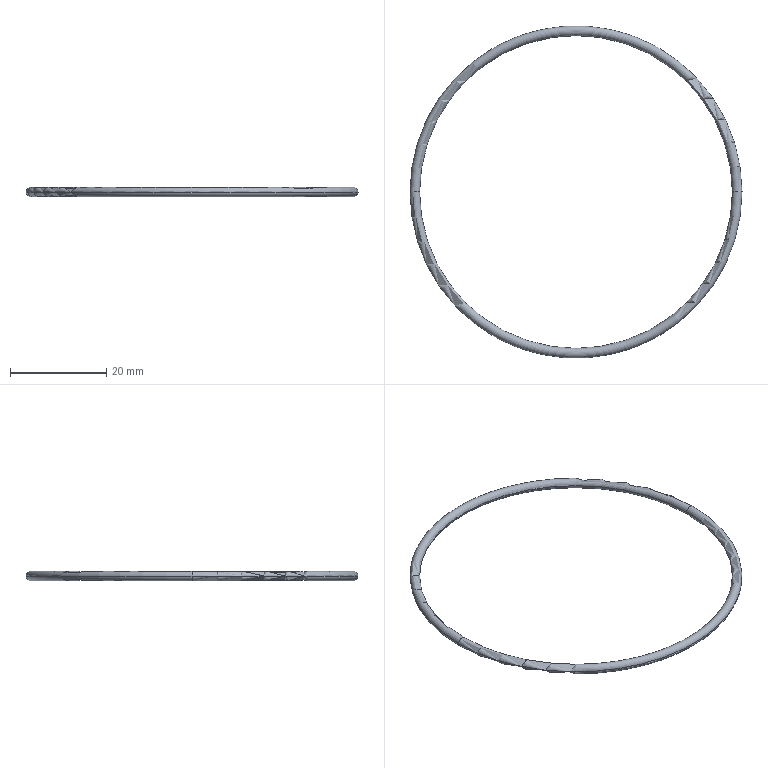Part | SolidWorks | features RefAxis 1, Revolution 1 | 1 solid | 4 faces | box 69 x 69 x 2 mm | volume 661.263 mm3 | torus 4
STEP:
#1=CARTESIAN_POINT('',(34.5,0.,0.));
#2=VERTEX_POINT('',#1);
#3=CARTESIAN_POINT('',(32.5,0.,0.));
#4=VERTEX_POINT('',#3);
#5=CARTESIAN_POINT('',(33.5,0.,0.));
#6=DIRECTION('',(0.,1.,0.));
#7=DIRECTION('',(-1.,0.,0.));
#8=AXIS2_PLACEMENT_3D('',#5,#6,#7);
#9=CIRCLE('',#8,1.);
#10=EDGE_CURVE('',#2,#4,#9,.T.);
#11=ORIENTED_EDGE('',*,*,#10,.F.);
#12=CARTESIAN_POINT('',(-34.5,0.,0.));
#13=VERTEX_POINT('',#12);
#14=CARTESIAN_POINT('',(0.,0.,0.));
#15=DIRECTION('',(0.,0.,-1.));
#16=DIRECTION('',(-1.,0.,0.));
#17=AXIS2_PLACEMENT_3D('',#14,#15,#16);
#18=CIRCLE('',#17,34.5);
#19=EDGE_CURVE('',#2,#13,#18,.T.);
#20=ORIENTED_EDGE('',*,*,#19,.T.);
#21=CARTESIAN_POINT('',(-32.5,0.,0.));
#22=VERTEX_POINT('',#21);
#23=CARTESIAN_POINT('',(-33.5,0.,0.));
#24=DIRECTION('',(0.,-1.,0.));
#25=DIRECTION('',(0.,0.,-1.));
#26=AXIS2_PLACEMENT_3D('',#23,#24,#25);
#27=CIRCLE('',#26,1.);
#28=EDGE_CURVE('',#13,#22,#27,.T.);
#29=ORIENTED_EDGE('',*,*,#28,.T.);
#30=CARTESIAN_POINT('',(0.,0.,0.));
#31=DIRECTION('',(0.,0.,-1.));
#32=DIRECTION('',(-1.,0.,0.));
#33=AXIS2_PLACEMENT_3D('',#30,#31,#32);
#34=CIRCLE('',#33,32.5);
#35=EDGE_CURVE('',#4,#22,#34,.T.);
#36=ORIENTED_EDGE('',*,*,#35,.F.);
#37=EDGE_LOOP('',(#11,#20,#29,#36));
#38=FACE_OUTER_BOUND('',#37,.T.);
#39=CARTESIAN_POINT('',(0.,0.,0.));
#40=DIRECTION('',(0.,0.,-1.));
#41=DIRECTION('',(-1.,0.,0.));
#42=AXIS2_PLACEMENT_3D('',#39,#40,#41);
#43=TOROIDAL_SURFACE('',#42,33.5,1.);
#44=ADVANCED_FACE('',(#38),#43,.T.);
#45=ORIENTED_EDGE('',*,*,#28,.F.);
#46=CARTESIAN_POINT('',(0.,0.,0.));
#47=DIRECTION('',(0.,0.,-1.));
#48=DIRECTION('',(-1.,0.,0.));
#49=AXIS2_PLACEMENT_3D('',#46,#47,#48);
#50=CIRCLE('',#49,34.5);
#51=EDGE_CURVE('',#13,#2,#50,.T.);
#52=ORIENTED_EDGE('',*,*,#51,.T.);
#53=ORIENTED_EDGE('',*,*,#10,.T.);
#54=CARTESIAN_POINT('',(0.,0.,0.));
#55=DIRECTION('',(0.,0.,-1.));
#56=DIRECTION('',(-1.,0.,0.));
#57=AXIS2_PLACEMENT_3D('',#54,#55,#56);
#58=CIRCLE('',#57,32.5);
#59=EDGE_CURVE('',#22,#4,#58,.T.);
#60=ORIENTED_EDGE('',*,*,#59,.F.);
#61=EDGE_LOOP('',(#45,#52,#53,#60));
#62=FACE_OUTER_BOUND('',#61,.T.);
#63=CARTESIAN_POINT('',(0.,0.,0.));
#64=DIRECTION('',(0.,0.,-1.));
#65=DIRECTION('',(-1.,0.,0.));
#66=AXIS2_PLACEMENT_3D('',#63,#64,#65);
#67=TOROIDAL_SURFACE('',#66,33.5,1.);
#68=ADVANCED_FACE('',(#62),#67,.T.);
#69=ORIENTED_EDGE('',*,*,#51,.F.);
#70=CARTESIAN_POINT('',(-33.5,0.,0.));
#71=DIRECTION('',(0.,-1.,0.));
#72=DIRECTION('',(0.,0.,-1.));
#73=AXIS2_PLACEMENT_3D('',#70,#71,#72);
#74=CIRCLE('',#73,1.);
#75=EDGE_CURVE('',#22,#13,#74,.T.);
#76=ORIENTED_EDGE('',*,*,#75,.F.);
#77=ORIENTED_EDGE('',*,*,#59,.T.);
#78=CARTESIAN_POINT('',(33.5,0.,0.));
#79=DIRECTION('',(0.,1.,0.));
#80=DIRECTION('',(-1.,0.,0.));
#81=AXIS2_PLACEMENT_3D('',#78,#79,#80);
#82=CIRCLE('',#81,1.);
#83=EDGE_CURVE('',#4,#2,#82,.T.);
#84=ORIENTED_EDGE('',*,*,#83,.T.);
#85=EDGE_LOOP('',(#69,#76,#77,#84));
#86=FACE_OUTER_BOUND('',#85,.T.);
#87=CARTESIAN_POINT('',(0.,0.,0.));
#88=DIRECTION('',(0.,0.,-1.));
#89=DIRECTION('',(-1.,0.,0.));
#90=AXIS2_PLACEMENT_3D('',#87,#88,#89);
#91=TOROIDAL_SURFACE('',#90,33.5,1.);
#92=ADVANCED_FACE('',(#86),#91,.T.);
#93=ORIENTED_EDGE('',*,*,#19,.F.);
#94=ORIENTED_EDGE('',*,*,#83,.F.);
#95=ORIENTED_EDGE('',*,*,#35,.T.);
#96=ORIENTED_EDGE('',*,*,#75,.T.);
#97=EDGE_LOOP('',(#93,#94,#95,#96));
#98=FACE_OUTER_BOUND('',#97,.T.);
#99=CARTESIAN_POINT('',(0.,0.,0.));
#100=DIRECTION('',(0.,0.,-1.));
#101=DIRECTION('',(-1.,0.,0.));
#102=AXIS2_PLACEMENT_3D('',#99,#100,#101);
#103=TOROIDAL_SURFACE('',#102,33.5,1.);
#104=ADVANCED_FACE('',(#98),#103,.T.);
#105=CLOSED_SHELL('',(#44,#68,#92,#104));
#106=MANIFOLD_SOLID_BREP('',#105);
#107=CARTESIAN_POINT('',(0.,0.,0.));
#108=DIRECTION('',(0.,0.,1.));
#109=DIRECTION('',(1.,0.,0.));
#110=AXIS2_PLACEMENT_3D('',#107,#108,#109);
#111=(LENGTH_UNIT()NAMED_UNIT(*)SI_UNIT(.MILLI.,.METRE.));
#112=UNCERTAINTY_MEASURE_WITH_UNIT(LENGTH_MEASURE(0.00001),#111,'','');
#113=(NAMED_UNIT(*)PLANE_ANGLE_UNIT()SI_UNIT($,.RADIAN.));
#114=(NAMED_UNIT(*)SI_UNIT($,.STERADIAN.)SOLID_ANGLE_UNIT());
#115=(GEOMETRIC_REPRESENTATION_CONTEXT(3)GLOBAL_UNCERTAINTY_ASSIGNED_CONTEXT((#112))GLOBAL_UNIT_ASSIGNED_CONTEXT((#111,#113,#114))REPRESENTATION_CONTEXT('',''));
#116=ADVANCED_BREP_SHAPE_REPRESENTATION('',(#106,#110),#115);